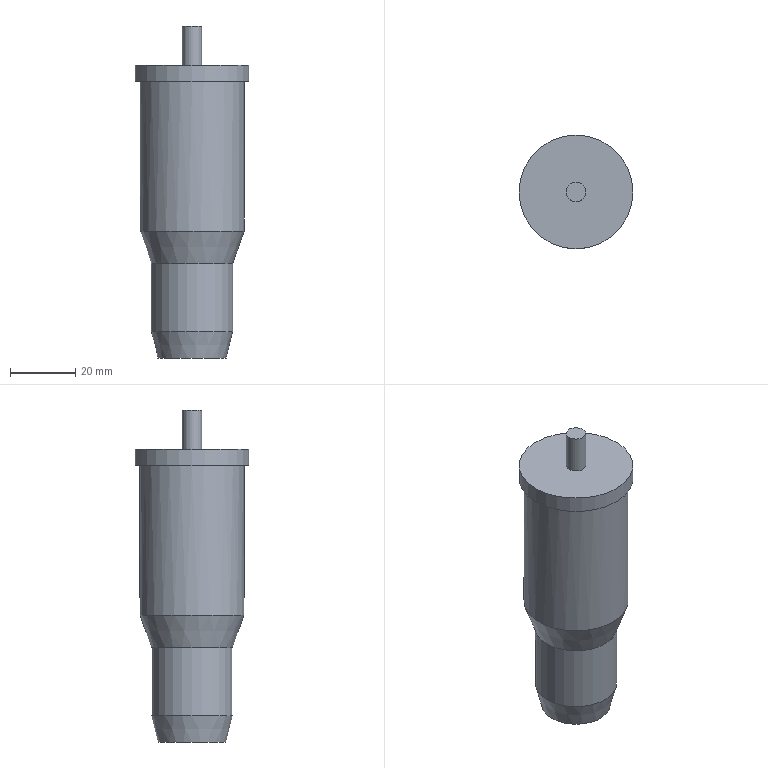Part | NX | features solid 2 | 1 solid | 10 faces | box 35 x 35 x 102 mm | volume 62197 mm3 | cylinder 4 | plane 4 | cone 2 | commonest cylinder face diameters 6 x1 25 x1 32 x1 35 x1
STEP:
#1=CARTESIAN_POINT('',(68.931,179.38,34.));
#2=VERTEX_POINT('',#1);
#3=CARTESIAN_POINT('',(56.431,179.38,34.));
#4=DIRECTION('',(0.,0.,1.));
#5=DIRECTION('',(1.,0.,0.));
#6=AXIS2_PLACEMENT_3D('',#3,#4,#5);
#7=CIRCLE('',#6,12.5);
#8=EDGE_CURVE('',#2,#2,#7,.T.);
#9=ORIENTED_EDGE('',*,*,#8,.F.);
#10=EDGE_LOOP('',(#9));
#11=FACE_BOUND('',#10,.T.);
#12=CARTESIAN_POINT('',(68.931,179.38,13.));
#13=VERTEX_POINT('',#12);
#14=CARTESIAN_POINT('',(56.431,179.38,13.));
#15=DIRECTION('',(0.,0.,1.));
#16=DIRECTION('',(1.,0.,0.));
#17=AXIS2_PLACEMENT_3D('',#14,#15,#16);
#18=CIRCLE('',#17,12.5);
#19=EDGE_CURVE('',#13,#13,#18,.T.);
#20=ORIENTED_EDGE('',*,*,#19,.T.);
#21=EDGE_LOOP('',(#20));
#22=FACE_BOUND('',#21,.T.);
#23=CARTESIAN_POINT('',(56.431,179.38,15.));
#24=DIRECTION('',(0.,0.,1.));
#25=DIRECTION('',(1.,0.,0.));
#26=AXIS2_PLACEMENT_3D('',#23,#24,#25);
#27=CYLINDRICAL_SURFACE('',#26,12.5);
#28=ADVANCED_FACE('',(#11,#22),#27,.T.);
#29=ORIENTED_EDGE('',*,*,#8,.T.);
#30=EDGE_LOOP('',(#29));
#31=FACE_BOUND('',#30,.T.);
#32=CARTESIAN_POINT('',(72.431,179.38,44.));
#33=VERTEX_POINT('',#32);
#34=CARTESIAN_POINT('',(56.431,179.38,44.));
#35=DIRECTION('',(0.,0.,1.));
#36=DIRECTION('',(1.,0.,0.));
#37=AXIS2_PLACEMENT_3D('',#34,#35,#36);
#38=CIRCLE('',#37,16.);
#39=EDGE_CURVE('',#33,#33,#38,.T.);
#40=ORIENTED_EDGE('',*,*,#39,.F.);
#41=EDGE_LOOP('',(#40));
#42=FACE_BOUND('',#41,.T.);
#43=CARTESIAN_POINT('',(56.431,179.38,34.));
#44=DIRECTION('',(0.,0.,1.));
#45=DIRECTION('',(1.,0.,0.));
#46=AXIS2_PLACEMENT_3D('',#43,#44,#45);
#47=CONICAL_SURFACE('',#46,12.5,0.3367);
#48=ADVANCED_FACE('',(#31,#42),#47,.T.);
#49=CARTESIAN_POINT('',(40.431,179.38,90.));
#50=VERTEX_POINT('',#49);
#51=CARTESIAN_POINT('',(56.431,179.38,90.));
#52=DIRECTION('',(0.,0.,-1.));
#53=DIRECTION('',(-1.,0.,0.));
#54=AXIS2_PLACEMENT_3D('',#51,#52,#53);
#55=CIRCLE('',#54,16.);
#56=EDGE_CURVE('',#50,#50,#55,.F.);
#57=ORIENTED_EDGE('',*,*,#56,.F.);
#58=EDGE_LOOP('',(#57));
#59=FACE_BOUND('',#58,.T.);
#60=ORIENTED_EDGE('',*,*,#39,.T.);
#61=EDGE_LOOP('',(#60));
#62=FACE_BOUND('',#61,.T.);
#63=CARTESIAN_POINT('',(56.431,179.38,44.));
#64=DIRECTION('',(0.,0.,1.));
#65=DIRECTION('',(1.,0.,0.));
#66=AXIS2_PLACEMENT_3D('',#63,#64,#65);
#67=CYLINDRICAL_SURFACE('',#66,16.);
#68=ADVANCED_FACE('',(#59,#62),#67,.T.);
#69=CARTESIAN_POINT('',(59.431,179.38,95.));
#70=VERTEX_POINT('',#69);
#71=CARTESIAN_POINT('',(56.431,179.38,95.));
#72=DIRECTION('',(0.,0.,1.));
#73=DIRECTION('',(1.,0.,0.));
#74=AXIS2_PLACEMENT_3D('',#71,#72,#73);
#75=CIRCLE('',#74,3.);
#76=EDGE_CURVE('',#70,#70,#75,.T.);
#77=ORIENTED_EDGE('',*,*,#76,.F.);
#78=EDGE_LOOP('',(#77));
#79=FACE_BOUND('',#78,.T.);
#80=CARTESIAN_POINT('',(38.931,179.38,95.));
#81=VERTEX_POINT('',#80);
#82=CARTESIAN_POINT('',(56.431,179.38,95.));
#83=DIRECTION('',(0.,0.,-1.));
#84=DIRECTION('',(-1.,0.,0.));
#85=AXIS2_PLACEMENT_3D('',#82,#83,#84);
#86=CIRCLE('',#85,17.5);
#87=EDGE_CURVE('',#81,#81,#86,.T.);
#88=ORIENTED_EDGE('',*,*,#87,.F.);
#89=EDGE_LOOP('',(#88));
#90=FACE_BOUND('',#89,.T.);
#91=CARTESIAN_POINT('',(56.431,179.38,95.));
#92=DIRECTION('',(0.,0.,1.));
#93=DIRECTION('',(1.,0.,0.));
#94=AXIS2_PLACEMENT_3D('',#91,#92,#93);
#95=PLANE('',#94);
#96=ADVANCED_FACE('',(#79,#90),#95,.T.);
#97=ORIENTED_EDGE('',*,*,#56,.T.);
#98=EDGE_LOOP('',(#97));
#99=FACE_BOUND('',#98,.T.);
#100=CARTESIAN_POINT('',(73.931,179.38,90.));
#101=VERTEX_POINT('',#100);
#102=CARTESIAN_POINT('',(56.431,179.38,90.));
#103=DIRECTION('',(0.,0.,1.));
#104=DIRECTION('',(1.,0.,0.));
#105=AXIS2_PLACEMENT_3D('',#102,#103,#104);
#106=CIRCLE('',#105,17.5);
#107=EDGE_CURVE('',#101,#101,#106,.T.);
#108=ORIENTED_EDGE('',*,*,#107,.F.);
#109=EDGE_LOOP('',(#108));
#110=FACE_BOUND('',#109,.T.);
#111=CARTESIAN_POINT('',(56.431,179.38,90.));
#112=DIRECTION('',(0.,0.,-1.));
#113=DIRECTION('',(-1.,0.,0.));
#114=AXIS2_PLACEMENT_3D('',#111,#112,#113);
#115=PLANE('',#114);
#116=ADVANCED_FACE('',(#99,#110),#115,.T.);
#117=ORIENTED_EDGE('',*,*,#87,.T.);
#118=EDGE_LOOP('',(#117));
#119=FACE_BOUND('',#118,.T.);
#120=ORIENTED_EDGE('',*,*,#107,.T.);
#121=EDGE_LOOP('',(#120));
#122=FACE_BOUND('',#121,.T.);
#123=CARTESIAN_POINT('',(56.431,179.38,90.));
#124=DIRECTION('',(0.,0.,1.));
#125=DIRECTION('',(1.,0.,0.));
#126=AXIS2_PLACEMENT_3D('',#123,#124,#125);
#127=CYLINDRICAL_SURFACE('',#126,17.5);
#128=ADVANCED_FACE('',(#119,#122),#127,.T.);
#129=CARTESIAN_POINT('',(53.431,179.38,107.));
#130=VERTEX_POINT('',#129);
#131=CARTESIAN_POINT('',(56.431,179.38,107.));
#132=DIRECTION('',(0.,0.,-1.));
#133=DIRECTION('',(-1.,0.,0.));
#134=AXIS2_PLACEMENT_3D('',#131,#132,#133);
#135=CIRCLE('',#134,3.);
#136=EDGE_CURVE('',#130,#130,#135,.T.);
#137=ORIENTED_EDGE('',*,*,#136,.F.);
#138=EDGE_LOOP('',(#137));
#139=FACE_BOUND('',#138,.T.);
#140=CARTESIAN_POINT('',(56.431,179.38,107.));
#141=DIRECTION('',(0.,0.,1.));
#142=DIRECTION('',(1.,0.,0.));
#143=AXIS2_PLACEMENT_3D('',#140,#141,#142);
#144=PLANE('',#143);
#145=ADVANCED_FACE('',(#139),#144,.T.);
#146=ORIENTED_EDGE('',*,*,#136,.T.);
#147=EDGE_LOOP('',(#146));
#148=FACE_BOUND('',#147,.T.);
#149=ORIENTED_EDGE('',*,*,#76,.T.);
#150=EDGE_LOOP('',(#149));
#151=FACE_BOUND('',#150,.T.);
#152=CARTESIAN_POINT('',(56.431,179.38,95.));
#153=DIRECTION('',(0.,0.,1.));
#154=DIRECTION('',(1.,0.,0.));
#155=AXIS2_PLACEMENT_3D('',#152,#153,#154);
#156=CYLINDRICAL_SURFACE('',#155,3.);
#157=ADVANCED_FACE('',(#148,#151),#156,.T.);
#158=CARTESIAN_POINT('',(45.931,179.38,5.));
#159=VERTEX_POINT('',#158);
#160=CARTESIAN_POINT('',(56.431,179.38,5.));
#161=DIRECTION('',(0.,0.,-1.));
#162=DIRECTION('',(-1.,0.,0.));
#163=AXIS2_PLACEMENT_3D('',#160,#161,#162);
#164=CIRCLE('',#163,10.5);
#165=EDGE_CURVE('',#159,#159,#164,.T.);
#166=ORIENTED_EDGE('',*,*,#165,.T.);
#167=EDGE_LOOP('',(#166));
#168=FACE_BOUND('',#167,.T.);
#169=CARTESIAN_POINT('',(56.431,179.38,5.));
#170=DIRECTION('',(0.,0.,-1.));
#171=DIRECTION('',(-1.,0.,0.));
#172=AXIS2_PLACEMENT_3D('',#169,#170,#171);
#173=PLANE('',#172);
#174=ADVANCED_FACE('',(#168),#173,.T.);
#175=ORIENTED_EDGE('',*,*,#165,.F.);
#176=EDGE_LOOP('',(#175));
#177=FACE_BOUND('',#176,.T.);
#178=ORIENTED_EDGE('',*,*,#19,.F.);
#179=EDGE_LOOP('',(#178));
#180=FACE_BOUND('',#179,.T.);
#181=CARTESIAN_POINT('',(56.431,179.38,13.));
#182=DIRECTION('',(0.,0.,1.));
#183=DIRECTION('',(1.,0.,0.));
#184=AXIS2_PLACEMENT_3D('',#181,#182,#183);
#185=CONICAL_SURFACE('',#184,12.5,0.245);
#186=ADVANCED_FACE('',(#177,#180),#185,.T.);
#187=CLOSED_SHELL('',(#28,#48,#68,#96,#116,#128,#145,#157,#174,#186));
#188=MANIFOLD_SOLID_BREP('',#187);
#189=(LENGTH_UNIT()NAMED_UNIT(*)SI_UNIT(.MILLI.,.METRE.));
#190=UNCERTAINTY_MEASURE_WITH_UNIT(LENGTH_MEASURE(0.00001),#189,'','');
#191=(NAMED_UNIT(*)PLANE_ANGLE_UNIT()SI_UNIT($,.RADIAN.));
#192=(NAMED_UNIT(*)SI_UNIT($,.STERADIAN.)SOLID_ANGLE_UNIT());
#193=(GEOMETRIC_REPRESENTATION_CONTEXT(3)GLOBAL_UNCERTAINTY_ASSIGNED_CONTEXT((#190))GLOBAL_UNIT_ASSIGNED_CONTEXT((#189,#191,#192))REPRESENTATION_CONTEXT('',''));
#194=ADVANCED_BREP_SHAPE_REPRESENTATION('',(#188),#193);